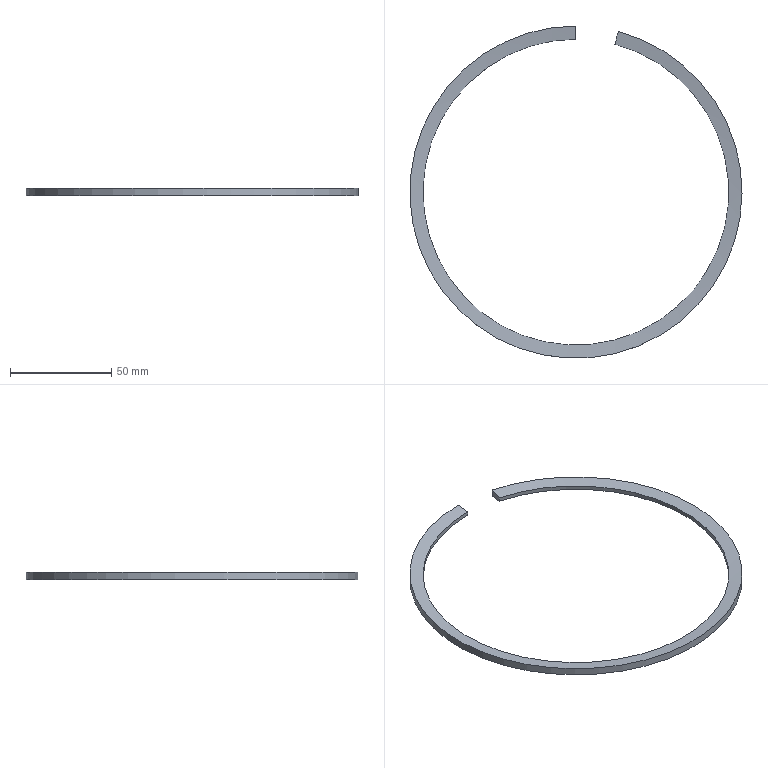Part | NX | features DATUM_CSYS 2, SKETCH 1, SWP104 1 | 1 solid | 6 faces | box 164 x 164 x 3.7 mm | volume 8808 mm3 | cylinder 2 | cone 2 | plane 2 | commonest cylinder face diameters 151 x1 164 x1
STEP:
#1=CARTESIAN_POINT('',(19.286,72.995,0.8557));
#2=VERTEX_POINT('',#1);
#3=CARTESIAN_POINT('',(0.,75.5,0.8557));
#4=VERTEX_POINT('',#3);
#5=CARTESIAN_POINT('',(0.,0.,0.8557));
#6=DIRECTION('',(0.,0.,-1.));
#7=DIRECTION('',(-1.,0.,0.));
#8=AXIS2_PLACEMENT_3D('',#5,#6,#7);
#9=CIRCLE('',#8,75.5);
#10=EDGE_CURVE('',#2,#4,#9,.T.);
#11=ORIENTED_EDGE('',*,*,#10,.T.);
#12=CARTESIAN_POINT('',(0.,75.5,2.844));
#13=VERTEX_POINT('',#12);
#14=CARTESIAN_POINT('',(0.,75.5,2.844));
#15=DIRECTION('',(0.,0.,-1.));
#16=VECTOR('',#15,1000.);
#17=LINE('',#14,#16);
#18=EDGE_CURVE('',#13,#4,#17,.T.);
#19=ORIENTED_EDGE('',*,*,#18,.F.);
#20=CARTESIAN_POINT('',(19.286,72.995,2.844));
#21=VERTEX_POINT('',#20);
#22=CARTESIAN_POINT('',(0.,0.,2.844));
#23=DIRECTION('',(0.,0.,-1.));
#24=DIRECTION('',(-1.,0.,0.));
#25=AXIS2_PLACEMENT_3D('',#22,#23,#24);
#26=CIRCLE('',#25,75.5);
#27=EDGE_CURVE('',#21,#13,#26,.T.);
#28=ORIENTED_EDGE('',*,*,#27,.F.);
#29=CARTESIAN_POINT('',(19.286,72.995,2.844));
#30=DIRECTION('',(0.,0.,-1.));
#31=VECTOR('',#30,1000.);
#32=LINE('',#29,#31);
#33=EDGE_CURVE('',#21,#2,#32,.T.);
#34=ORIENTED_EDGE('',*,*,#33,.T.);
#35=EDGE_LOOP('',(#11,#19,#28,#34));
#36=FACE_BOUND('',#35,.T.);
#37=CARTESIAN_POINT('',(0.,0.,0.));
#38=DIRECTION('',(0.,0.,-1.));
#39=DIRECTION('',(-1.,0.,0.));
#40=AXIS2_PLACEMENT_3D('',#37,#38,#39);
#41=CYLINDRICAL_SURFACE('',#40,75.5);
#42=ADVANCED_FACE('',(#36),#41,.F.);
#43=CARTESIAN_POINT('',(20.947,79.28,0.));
#44=VERTEX_POINT('',#43);
#45=CARTESIAN_POINT('',(0.,82.,0.));
#46=VERTEX_POINT('',#45);
#47=CARTESIAN_POINT('',(0.,0.,0.));
#48=DIRECTION('',(0.,0.,-1.));
#49=DIRECTION('',(-1.,0.,0.));
#50=AXIS2_PLACEMENT_3D('',#47,#48,#49);
#51=CIRCLE('',#50,82.);
#52=EDGE_CURVE('',#44,#46,#51,.T.);
#53=ORIENTED_EDGE('',*,*,#52,.T.);
#54=CARTESIAN_POINT('',(0.,75.5,0.8557));
#55=DIRECTION('',(0.,0.9914,-0.1305));
#56=VECTOR('',#55,1000.);
#57=LINE('',#54,#56);
#58=EDGE_CURVE('',#4,#46,#57,.T.);
#59=ORIENTED_EDGE('',*,*,#58,.F.);
#60=ORIENTED_EDGE('',*,*,#10,.F.);
#61=CARTESIAN_POINT('',(19.286,72.995,0.8557));
#62=DIRECTION('',(0.2533,0.9586,-0.1305));
#63=VECTOR('',#62,1000.);
#64=LINE('',#61,#63);
#65=EDGE_CURVE('',#2,#44,#64,.T.);
#66=ORIENTED_EDGE('',*,*,#65,.T.);
#67=EDGE_LOOP('',(#53,#59,#60,#66));
#68=FACE_BOUND('',#67,.T.);
#69=CARTESIAN_POINT('',(0.,0.,0.8557));
#70=DIRECTION('',(0.,0.,-1.));
#71=DIRECTION('',(-1.,0.,0.));
#72=AXIS2_PLACEMENT_3D('',#69,#70,#71);
#73=CONICAL_SURFACE('',#72,75.5,1.44);
#74=ADVANCED_FACE('',(#68),#73,.F.);
#75=CARTESIAN_POINT('',(20.947,79.28,3.7));
#76=VERTEX_POINT('',#75);
#77=CARTESIAN_POINT('',(0.,82.,3.7));
#78=VERTEX_POINT('',#77);
#79=CARTESIAN_POINT('',(0.,0.,3.7));
#80=DIRECTION('',(0.,0.,-1.));
#81=DIRECTION('',(-1.,0.,0.));
#82=AXIS2_PLACEMENT_3D('',#79,#80,#81);
#83=CIRCLE('',#82,82.);
#84=EDGE_CURVE('',#76,#78,#83,.T.);
#85=ORIENTED_EDGE('',*,*,#84,.T.);
#86=CARTESIAN_POINT('',(0.,82.,0.));
#87=DIRECTION('',(0.,0.,1.));
#88=VECTOR('',#87,1000.);
#89=LINE('',#86,#88);
#90=EDGE_CURVE('',#46,#78,#89,.T.);
#91=ORIENTED_EDGE('',*,*,#90,.F.);
#92=ORIENTED_EDGE('',*,*,#52,.F.);
#93=CARTESIAN_POINT('',(20.947,79.28,0.));
#94=DIRECTION('',(0.,0.,1.));
#95=VECTOR('',#94,1000.);
#96=LINE('',#93,#95);
#97=EDGE_CURVE('',#44,#76,#96,.T.);
#98=ORIENTED_EDGE('',*,*,#97,.T.);
#99=EDGE_LOOP('',(#85,#91,#92,#98));
#100=FACE_BOUND('',#99,.T.);
#101=CARTESIAN_POINT('',(0.,0.,0.));
#102=DIRECTION('',(0.,0.,-1.));
#103=DIRECTION('',(-1.,0.,0.));
#104=AXIS2_PLACEMENT_3D('',#101,#102,#103);
#105=CYLINDRICAL_SURFACE('',#104,82.);
#106=ADVANCED_FACE('',(#100),#105,.T.);
#107=CARTESIAN_POINT('',(20.947,79.28,3.7));
#108=DIRECTION('',(-0.2533,-0.9586,-0.1305));
#109=VECTOR('',#108,1000.);
#110=LINE('',#107,#109);
#111=EDGE_CURVE('',#76,#21,#110,.T.);
#112=ORIENTED_EDGE('',*,*,#111,.T.);
#113=ORIENTED_EDGE('',*,*,#27,.T.);
#114=CARTESIAN_POINT('',(0.,82.,3.7));
#115=DIRECTION('',(0.,-0.9914,-0.1305));
#116=VECTOR('',#115,1000.);
#117=LINE('',#114,#116);
#118=EDGE_CURVE('',#78,#13,#117,.T.);
#119=ORIENTED_EDGE('',*,*,#118,.F.);
#120=ORIENTED_EDGE('',*,*,#84,.F.);
#121=EDGE_LOOP('',(#112,#113,#119,#120));
#122=FACE_BOUND('',#121,.T.);
#123=CARTESIAN_POINT('',(0.,0.,3.7));
#124=DIRECTION('',(0.,0.,1.));
#125=DIRECTION('',(1.,0.,0.));
#126=AXIS2_PLACEMENT_3D('',#123,#124,#125);
#127=CONICAL_SURFACE('',#126,82.,1.44);
#128=ADVANCED_FACE('',(#122),#127,.F.);
#129=ORIENTED_EDGE('',*,*,#33,.F.);
#130=ORIENTED_EDGE('',*,*,#111,.F.);
#131=ORIENTED_EDGE('',*,*,#97,.F.);
#132=ORIENTED_EDGE('',*,*,#65,.F.);
#133=EDGE_LOOP('',(#129,#130,#131,#132));
#134=FACE_BOUND('',#133,.T.);
#135=CARTESIAN_POINT('',(0.,0.,0.));
#136=DIRECTION('',(0.9668,-0.2554,0.));
#137=DIRECTION('',(0.,0.,-1.));
#138=AXIS2_PLACEMENT_3D('',#135,#136,#137);
#139=PLANE('',#138);
#140=ADVANCED_FACE('',(#134),#139,.F.);
#141=ORIENTED_EDGE('',*,*,#18,.T.);
#142=ORIENTED_EDGE('',*,*,#58,.T.);
#143=ORIENTED_EDGE('',*,*,#90,.T.);
#144=ORIENTED_EDGE('',*,*,#118,.T.);
#145=EDGE_LOOP('',(#141,#142,#143,#144));
#146=FACE_BOUND('',#145,.T.);
#147=CARTESIAN_POINT('',(0.,0.,0.));
#148=DIRECTION('',(1.,0.,0.));
#149=DIRECTION('',(0.,0.,-1.));
#150=AXIS2_PLACEMENT_3D('',#147,#148,#149);
#151=PLANE('',#150);
#152=ADVANCED_FACE('',(#146),#151,.T.);
#153=CLOSED_SHELL('',(#42,#74,#106,#128,#140,#152));
#154=MANIFOLD_SOLID_BREP('',#153);
#155=(LENGTH_UNIT()NAMED_UNIT(*)SI_UNIT(.MILLI.,.METRE.));
#156=UNCERTAINTY_MEASURE_WITH_UNIT(LENGTH_MEASURE(0.00001),#155,'','');
#157=(NAMED_UNIT(*)PLANE_ANGLE_UNIT()SI_UNIT($,.RADIAN.));
#158=(NAMED_UNIT(*)SI_UNIT($,.STERADIAN.)SOLID_ANGLE_UNIT());
#159=(GEOMETRIC_REPRESENTATION_CONTEXT(3)GLOBAL_UNCERTAINTY_ASSIGNED_CONTEXT((#156))GLOBAL_UNIT_ASSIGNED_CONTEXT((#155,#157,#158))REPRESENTATION_CONTEXT('',''));
#160=ADVANCED_BREP_SHAPE_REPRESENTATION('',(#154),#159);